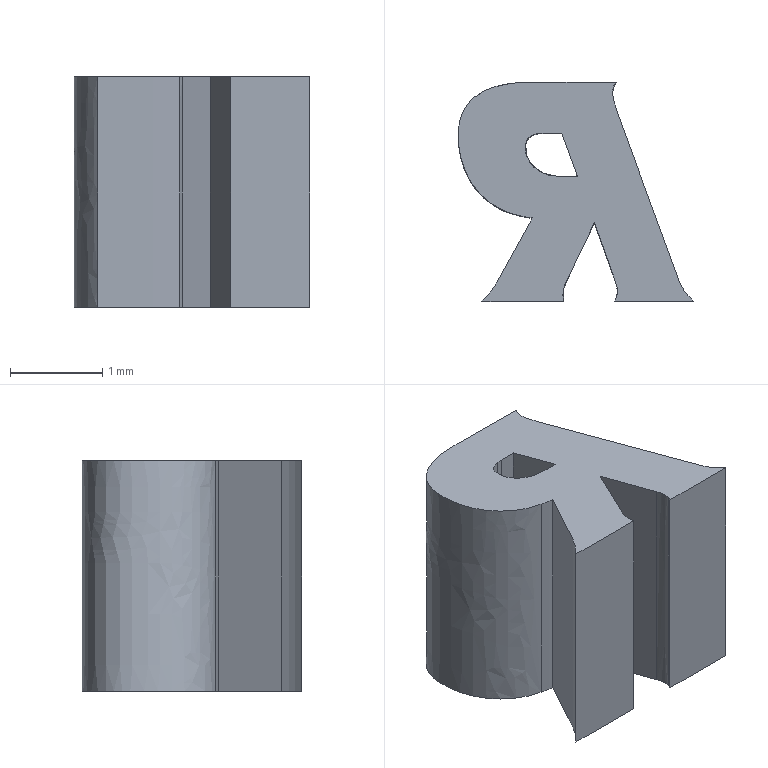Part | STEP file | lll_id1154_x_t | 1 solid | 23 faces | box 2.566 x 2.385 x 2.5 mm | volume 9.126 mm3 | plane 11 | other 7 | cylinder 5 | commonest cylinder face diameters 0.402 x1 1.036 x1 1.606 x1 2.67 x1 71.248 x1
STEP:
#1=CARTESIAN_POINT('',(384.184,124.408,2.35));
#2=VERTEX_POINT('',#1);
#3=CARTESIAN_POINT('',(384.356,123.934,2.35));
#4=VERTEX_POINT('',#3);
#5=CARTESIAN_POINT('',(384.356,123.934,2.35));
#6=DIRECTION('',(0.3416,-0.9399,0.));
#7=VECTOR('',#6,1.);
#8=LINE('',#5,#7);
#9=EDGE_CURVE('',#2,#4,#8,.T.);
#10=ORIENTED_EDGE('',*,*,#9,.F.);
#11=CARTESIAN_POINT('',(384.184,124.408,-0.15));
#12=VERTEX_POINT('',#11);
#13=CARTESIAN_POINT('',(384.184,124.408,-0.15));
#14=DIRECTION('',(0.,0.,-1.));
#15=VECTOR('',#14,1.);
#16=LINE('',#13,#15);
#17=EDGE_CURVE('',#2,#12,#16,.T.);
#18=ORIENTED_EDGE('',*,*,#17,.T.);
#19=CARTESIAN_POINT('',(384.356,123.934,-0.15));
#20=VERTEX_POINT('',#19);
#21=CARTESIAN_POINT('',(384.356,123.934,-0.15));
#22=DIRECTION('',(0.3416,-0.9399,0.));
#23=VECTOR('',#22,1.);
#24=LINE('',#21,#23);
#25=EDGE_CURVE('',#12,#20,#24,.T.);
#26=ORIENTED_EDGE('',*,*,#25,.T.);
#27=CARTESIAN_POINT('',(384.356,123.934,-0.15));
#28=DIRECTION('',(0.,0.,-1.));
#29=VECTOR('',#28,1.);
#30=LINE('',#27,#29);
#31=EDGE_CURVE('',#4,#20,#30,.T.);
#32=ORIENTED_EDGE('',*,*,#31,.F.);
#33=EDGE_LOOP('',(#10,#18,#26,#32));
#34=FACE_OUTER_BOUND('',#33,.T.);
#35=CARTESIAN_POINT('',(384.356,123.934,-0.15));
#36=DIRECTION('',(0.9399,0.3416,0.));
#37=DIRECTION('',(0.3416,-0.9399,0.));
#38=AXIS2_PLACEMENT_3D('',#35,#36,#37);
#39=PLANE('',#38);
#40=ADVANCED_FACE('',(#34),#39,.F.);
#41=CARTESIAN_POINT('',(383.996,124.408,2.35));
#42=VERTEX_POINT('',#41);
#43=CARTESIAN_POINT('',(384.184,124.408,2.35));
#44=DIRECTION('',(1.,0.,0.));
#45=VECTOR('',#44,1.);
#46=LINE('',#43,#45);
#47=EDGE_CURVE('',#42,#2,#46,.T.);
#48=ORIENTED_EDGE('',*,*,#47,.F.);
#49=CARTESIAN_POINT('',(383.996,124.408,-0.15));
#50=VERTEX_POINT('',#49);
#51=CARTESIAN_POINT('',(383.996,124.408,-0.15));
#52=DIRECTION('',(0.,0.,-1.));
#53=VECTOR('',#52,1.);
#54=LINE('',#51,#53);
#55=EDGE_CURVE('',#42,#50,#54,.T.);
#56=ORIENTED_EDGE('',*,*,#55,.T.);
#57=CARTESIAN_POINT('',(384.184,124.408,-0.15));
#58=DIRECTION('',(1.,0.,0.));
#59=VECTOR('',#58,1.);
#60=LINE('',#57,#59);
#61=EDGE_CURVE('',#50,#12,#60,.T.);
#62=ORIENTED_EDGE('',*,*,#61,.T.);
#63=ORIENTED_EDGE('',*,*,#17,.F.);
#64=EDGE_LOOP('',(#48,#56,#62,#63));
#65=FACE_OUTER_BOUND('',#64,.T.);
#66=CARTESIAN_POINT('',(384.184,124.408,-0.15));
#67=DIRECTION('',(0.,1.,0.));
#68=DIRECTION('',(0.,0.,1.));
#69=AXIS2_PLACEMENT_3D('',#66,#67,#68);
#70=PLANE('',#69);
#71=ADVANCED_FACE('',(#65),#70,.F.);
#72=CARTESIAN_POINT('',(383.942,124.405,2.35));
#73=VERTEX_POINT('',#72);
#74=CARTESIAN_POINT('',(383.942,124.405,2.35));
#75=CARTESIAN_POINT('',(383.951,124.406,2.35));
#76=CARTESIAN_POINT('',(383.96,124.407,2.35));
#77=CARTESIAN_POINT('',(383.978,124.408,2.35));
#78=CARTESIAN_POINT('',(383.987,124.408,2.35));
#79=CARTESIAN_POINT('',(383.996,124.408,2.35));
#80=(BOUNDED_CURVE()B_SPLINE_CURVE(3,(#74,#75,#76,#77,#78,#79),.UNSPECIFIED.,.F.,.F.)B_SPLINE_CURVE_WITH_KNOTS((4,2,4),(0.,0.5003,1.),.UNSPECIFIED.)CURVE()GEOMETRIC_REPRESENTATION_ITEM()RATIONAL_B_SPLINE_CURVE((0.5,0.4999,0.4999,0.5,0.5,0.5))REPRESENTATION_ITEM(''));
#81=EDGE_CURVE('',#73,#42,#80,.T.);
#82=ORIENTED_EDGE('',*,*,#81,.F.);
#83=CARTESIAN_POINT('',(383.942,124.405,-0.15));
#84=VERTEX_POINT('',#83);
#85=CARTESIAN_POINT('',(383.942,124.405,-0.15));
#86=DIRECTION('',(0.,0.,-1.));
#87=VECTOR('',#86,1.);
#88=LINE('',#85,#87);
#89=EDGE_CURVE('',#73,#84,#88,.T.);
#90=ORIENTED_EDGE('',*,*,#89,.T.);
#91=CARTESIAN_POINT('',(383.942,124.405,-0.15));
#92=CARTESIAN_POINT('',(383.951,124.406,-0.15));
#93=CARTESIAN_POINT('',(383.96,124.407,-0.15));
#94=CARTESIAN_POINT('',(383.978,124.408,-0.15));
#95=CARTESIAN_POINT('',(383.987,124.408,-0.15));
#96=CARTESIAN_POINT('',(383.996,124.408,-0.15));
#97=(BOUNDED_CURVE()B_SPLINE_CURVE(3,(#91,#92,#93,#94,#95,#96),.UNSPECIFIED.,.F.,.F.)B_SPLINE_CURVE_WITH_KNOTS((4,2,4),(0.,0.5003,1.),.UNSPECIFIED.)CURVE()GEOMETRIC_REPRESENTATION_ITEM()RATIONAL_B_SPLINE_CURVE((0.5,0.4999,0.4999,0.5,0.5,0.5))REPRESENTATION_ITEM(''));
#98=EDGE_CURVE('',#84,#50,#97,.T.);
#99=ORIENTED_EDGE('',*,*,#98,.T.);
#100=ORIENTED_EDGE('',*,*,#55,.F.);
#101=EDGE_LOOP('',(#82,#90,#99,#100));
#102=FACE_OUTER_BOUND('',#101,.T.);
#103=CARTESIAN_POINT('',(383.996,124.408,-0.15));
#104=CARTESIAN_POINT('',(383.987,124.408,-0.15));
#105=CARTESIAN_POINT('',(383.978,124.408,-0.15));
#106=CARTESIAN_POINT('',(383.96,124.407,-0.15));
#107=CARTESIAN_POINT('',(383.951,124.406,-0.15));
#108=CARTESIAN_POINT('',(383.942,124.405,-0.15));
#109=(BOUNDED_CURVE()B_SPLINE_CURVE(3,(#103,#104,#105,#106,#107,#108),.UNSPECIFIED.,.F.,.F.)B_SPLINE_CURVE_WITH_KNOTS((4,2,4),(0.,0.4997,1.),.UNSPECIFIED.)CURVE()GEOMETRIC_REPRESENTATION_ITEM()RATIONAL_B_SPLINE_CURVE((0.5,0.5,0.5,0.4999,0.4999,0.5))REPRESENTATION_ITEM(''));
#110=DIRECTION('',(0.,0.,1.));
#111=VECTOR('',#110,1.);
#112=SURFACE_OF_LINEAR_EXTRUSION('',#109,#111);
#113=ADVANCED_FACE('',(#102),#112,.F.);
#114=CARTESIAN_POINT('',(383.826,124.357,2.35));
#115=VERTEX_POINT('',#114);
#116=CARTESIAN_POINT('',(383.826,124.357,2.35));
#117=CARTESIAN_POINT('',(383.841,124.371,2.35));
#118=CARTESIAN_POINT('',(383.858,124.382,2.35));
#119=CARTESIAN_POINT('',(383.898,124.398,2.35));
#120=CARTESIAN_POINT('',(383.919,124.403,2.35));
#121=CARTESIAN_POINT('',(383.942,124.405,2.35));
#122=(BOUNDED_CURVE()B_SPLINE_CURVE(3,(#116,#117,#118,#119,#120,#121),.UNSPECIFIED.,.F.,.F.)B_SPLINE_CURVE_WITH_KNOTS((4,2,4),(0.,0.4721,1.),.UNSPECIFIED.)CURVE()GEOMETRIC_REPRESENTATION_ITEM()RATIONAL_B_SPLINE_CURVE((0.5,0.4937,0.4937,0.4969,0.4969,0.5))REPRESENTATION_ITEM(''));
#123=EDGE_CURVE('',#115,#73,#122,.T.);
#124=ORIENTED_EDGE('',*,*,#123,.F.);
#125=CARTESIAN_POINT('',(383.826,124.357,-0.15));
#126=VERTEX_POINT('',#125);
#127=CARTESIAN_POINT('',(383.826,124.357,-0.15));
#128=DIRECTION('',(0.,0.,-1.));
#129=VECTOR('',#128,1.);
#130=LINE('',#127,#129);
#131=EDGE_CURVE('',#115,#126,#130,.T.);
#132=ORIENTED_EDGE('',*,*,#131,.T.);
#133=CARTESIAN_POINT('',(383.826,124.357,-0.15));
#134=CARTESIAN_POINT('',(383.841,124.371,-0.15));
#135=CARTESIAN_POINT('',(383.858,124.382,-0.15));
#136=CARTESIAN_POINT('',(383.898,124.398,-0.15));
#137=CARTESIAN_POINT('',(383.919,124.403,-0.15));
#138=CARTESIAN_POINT('',(383.942,124.405,-0.15));
#139=(BOUNDED_CURVE()B_SPLINE_CURVE(3,(#133,#134,#135,#136,#137,#138),.UNSPECIFIED.,.F.,.F.)B_SPLINE_CURVE_WITH_KNOTS((4,2,4),(0.,0.4721,1.),.UNSPECIFIED.)CURVE()GEOMETRIC_REPRESENTATION_ITEM()RATIONAL_B_SPLINE_CURVE((0.5,0.4937,0.4937,0.4969,0.4969,0.5))REPRESENTATION_ITEM(''));
#140=EDGE_CURVE('',#126,#84,#139,.T.);
#141=ORIENTED_EDGE('',*,*,#140,.T.);
#142=ORIENTED_EDGE('',*,*,#89,.F.);
#143=EDGE_LOOP('',(#124,#132,#141,#142));
#144=FACE_OUTER_BOUND('',#143,.T.);
#145=CARTESIAN_POINT('',(383.942,124.405,-0.15));
#146=CARTESIAN_POINT('',(383.919,124.403,-0.15));
#147=CARTESIAN_POINT('',(383.898,124.398,-0.15));
#148=CARTESIAN_POINT('',(383.858,124.382,-0.15));
#149=CARTESIAN_POINT('',(383.841,124.371,-0.15));
#150=CARTESIAN_POINT('',(383.826,124.357,-0.15));
#151=(BOUNDED_CURVE()B_SPLINE_CURVE(3,(#145,#146,#147,#148,#149,#150),.UNSPECIFIED.,.F.,.F.)B_SPLINE_CURVE_WITH_KNOTS((4,2,4),(0.,0.5279,1.),.UNSPECIFIED.)CURVE()GEOMETRIC_REPRESENTATION_ITEM()RATIONAL_B_SPLINE_CURVE((0.5,0.4969,0.4969,0.4937,0.4937,0.5))REPRESENTATION_ITEM(''));
#152=DIRECTION('',(0.,0.,1.));
#153=VECTOR('',#152,1.);
#154=SURFACE_OF_LINEAR_EXTRUSION('',#151,#153);
#155=ADVANCED_FACE('',(#144),#154,.F.);
#156=CARTESIAN_POINT('',(384.178,123.934,2.35));
#157=VERTEX_POINT('',#156);
#158=CARTESIAN_POINT('',(384.178,123.934,2.35));
#159=CARTESIAN_POINT('',(384.16,123.934,2.35));
#160=CARTESIAN_POINT('',(384.142,123.935,2.35));
#161=CARTESIAN_POINT('',(384.102,123.939,2.35));
#162=CARTESIAN_POINT('',(384.08,123.942,2.35));
#163=CARTESIAN_POINT('',(384.032,123.953,2.35));
#164=CARTESIAN_POINT('',(384.007,123.961,2.35));
#165=CARTESIAN_POINT('',(383.945,123.988,2.35));
#166=CARTESIAN_POINT('',(383.912,124.01,2.35));
#167=CARTESIAN_POINT('',(383.842,124.074,2.35));
#168=CARTESIAN_POINT('',(383.814,124.121,2.35));
#169=CARTESIAN_POINT('',(383.791,124.199,2.35));
#170=CARTESIAN_POINT('',(383.787,124.225,2.35));
#171=CARTESIAN_POINT('',(383.787,124.268,2.35));
#172=CARTESIAN_POINT('',(383.789,124.284,2.35));
#173=CARTESIAN_POINT('',(383.799,124.321,2.35));
#174=CARTESIAN_POINT('',(383.81,124.341,2.35));
#175=CARTESIAN_POINT('',(383.826,124.357,2.35));
#176=(BOUNDED_CURVE()B_SPLINE_CURVE(3,(#158,#159,#160,#161,#162,#163,#164,#165,#166,#167,#168,#169,#170,#171,#172,#173,#174,#175),.UNSPECIFIED.,.F.,.F.)B_SPLINE_CURVE_WITH_KNOTS((4,2,2,2,2,2,2,2,4),(0.,0.07697,0.1735,0.2892,0.4651,0.7036,0.825,0.8964,1.),.UNSPECIFIED.)CURVE()GEOMETRIC_REPRESENTATION_ITEM()RATIONAL_B_SPLINE_CURVE((0.5,0.4998,0.4998,0.4994,0.4994,0.4983,0.4983,0.4952,0.4952,0.4878,0.4878,0.4966,0.4966,0.4974,0.4974,0.4878,0.4878,0.5))REPRESENTATION_ITEM(''));
#177=EDGE_CURVE('',#157,#115,#176,.T.);
#178=ORIENTED_EDGE('',*,*,#177,.F.);
#179=CARTESIAN_POINT('',(384.178,123.934,-0.15));
#180=VERTEX_POINT('',#179);
#181=CARTESIAN_POINT('',(384.178,123.934,-0.15));
#182=DIRECTION('',(0.,0.,-1.));
#183=VECTOR('',#182,1.);
#184=LINE('',#181,#183);
#185=EDGE_CURVE('',#157,#180,#184,.T.);
#186=ORIENTED_EDGE('',*,*,#185,.T.);
#187=CARTESIAN_POINT('',(384.178,123.934,-0.15));
#188=CARTESIAN_POINT('',(384.16,123.934,-0.15));
#189=CARTESIAN_POINT('',(384.142,123.935,-0.15));
#190=CARTESIAN_POINT('',(384.102,123.939,-0.15));
#191=CARTESIAN_POINT('',(384.08,123.942,-0.15));
#192=CARTESIAN_POINT('',(384.032,123.953,-0.15));
#193=CARTESIAN_POINT('',(384.007,123.961,-0.15));
#194=CARTESIAN_POINT('',(383.945,123.988,-0.15));
#195=CARTESIAN_POINT('',(383.912,124.01,-0.15));
#196=CARTESIAN_POINT('',(383.842,124.074,-0.15));
#197=CARTESIAN_POINT('',(383.814,124.121,-0.15));
#198=CARTESIAN_POINT('',(383.791,124.199,-0.15));
#199=CARTESIAN_POINT('',(383.787,124.225,-0.15));
#200=CARTESIAN_POINT('',(383.787,124.268,-0.15));
#201=CARTESIAN_POINT('',(383.789,124.284,-0.15));
#202=CARTESIAN_POINT('',(383.799,124.321,-0.15));
#203=CARTESIAN_POINT('',(383.81,124.341,-0.15));
#204=CARTESIAN_POINT('',(383.826,124.357,-0.15));
#205=(BOUNDED_CURVE()B_SPLINE_CURVE(3,(#187,#188,#189,#190,#191,#192,#193,#194,#195,#196,#197,#198,#199,#200,#201,#202,#203,#204),.UNSPECIFIED.,.F.,.F.)B_SPLINE_CURVE_WITH_KNOTS((4,2,2,2,2,2,2,2,4),(0.,0.07697,0.1735,0.2892,0.4651,0.7036,0.825,0.8964,1.),.UNSPECIFIED.)CURVE()GEOMETRIC_REPRESENTATION_ITEM()RATIONAL_B_SPLINE_CURVE((0.5,0.4998,0.4998,0.4994,0.4994,0.4983,0.4983,0.4952,0.4952,0.4878,0.4878,0.4966,0.4966,0.4974,0.4974,0.4878,0.4878,0.5))REPRESENTATION_ITEM(''));
#206=EDGE_CURVE('',#180,#126,#205,.T.);
#207=ORIENTED_EDGE('',*,*,#206,.T.);
#208=ORIENTED_EDGE('',*,*,#131,.F.);
#209=EDGE_LOOP('',(#178,#186,#207,#208));
#210=FACE_OUTER_BOUND('',#209,.T.);
#211=CARTESIAN_POINT('',(383.826,124.357,-0.15));
#212=CARTESIAN_POINT('',(383.81,124.341,-0.15));
#213=CARTESIAN_POINT('',(383.799,124.321,-0.15));
#214=CARTESIAN_POINT('',(383.789,124.284,-0.15));
#215=CARTESIAN_POINT('',(383.787,124.268,-0.15));
#216=CARTESIAN_POINT('',(383.787,124.225,-0.15));
#217=CARTESIAN_POINT('',(383.791,124.199,-0.15));
#218=CARTESIAN_POINT('',(383.814,124.121,-0.15));
#219=CARTESIAN_POINT('',(383.842,124.074,-0.15));
#220=CARTESIAN_POINT('',(383.912,124.01,-0.15));
#221=CARTESIAN_POINT('',(383.945,123.988,-0.15));
#222=CARTESIAN_POINT('',(384.007,123.961,-0.15));
#223=CARTESIAN_POINT('',(384.032,123.953,-0.15));
#224=CARTESIAN_POINT('',(384.08,123.942,-0.15));
#225=CARTESIAN_POINT('',(384.102,123.939,-0.15));
#226=CARTESIAN_POINT('',(384.142,123.935,-0.15));
#227=CARTESIAN_POINT('',(384.16,123.934,-0.15));
#228=CARTESIAN_POINT('',(384.178,123.934,-0.15));
#229=(BOUNDED_CURVE()B_SPLINE_CURVE(3,(#211,#212,#213,#214,#215,#216,#217,#218,#219,#220,#221,#222,#223,#224,#225,#226,#227,#228),.UNSPECIFIED.,.F.,.F.)B_SPLINE_CURVE_WITH_KNOTS((4,2,2,2,2,2,2,2,4),(0.,0.1036,0.175,0.2964,0.5349,0.7108,0.8265,0.923,1.),.UNSPECIFIED.)CURVE()GEOMETRIC_REPRESENTATION_ITEM()RATIONAL_B_SPLINE_CURVE((0.5,0.4878,0.4878,0.4974,0.4974,0.4966,0.4966,0.4878,0.4878,0.4952,0.4952,0.4983,0.4983,0.4994,0.4994,0.4998,0.4998,0.5))REPRESENTATION_ITEM(''));
#230=DIRECTION('',(0.,0.,1.));
#231=VECTOR('',#230,1.);
#232=SURFACE_OF_LINEAR_EXTRUSION('',#229,#231);
#233=ADVANCED_FACE('',(#210),#232,.F.);
#234=CARTESIAN_POINT('',(385.618,122.58,2.35));
#235=VERTEX_POINT('',#234);
#236=CARTESIAN_POINT('',(385.461,122.794,2.35));
#237=VERTEX_POINT('',#236);
#238=CARTESIAN_POINT('',(385.942,122.987,2.35));
#239=DIRECTION('',(0.,0.,-1.));
#240=DIRECTION('',(-1.,0.,0.));
#241=AXIS2_PLACEMENT_3D('',#238,#239,#240);
#242=CIRCLE('',#241,0.5179);
#243=EDGE_CURVE('',#235,#237,#242,.T.);
#244=ORIENTED_EDGE('',*,*,#243,.F.);
#245=CARTESIAN_POINT('',(385.618,122.58,-0.15));
#246=VERTEX_POINT('',#245);
#247=CARTESIAN_POINT('',(385.624,122.578,2.35));
#248=DIRECTION('',(0.,0.,-1.));
#249=VECTOR('',#248,1.);
#250=LINE('',#247,#249);
#251=EDGE_CURVE('',#235,#246,#250,.T.);
#252=ORIENTED_EDGE('',*,*,#251,.T.);
#253=CARTESIAN_POINT('',(385.461,122.794,-0.15));
#254=VERTEX_POINT('',#253);
#255=CARTESIAN_POINT('',(385.942,122.987,-0.15));
#256=DIRECTION('',(0.,0.,-1.));
#257=DIRECTION('',(-1.,0.,0.));
#258=AXIS2_PLACEMENT_3D('',#255,#256,#257);
#259=CIRCLE('',#258,0.5179);
#260=EDGE_CURVE('',#246,#254,#259,.T.);
#261=ORIENTED_EDGE('',*,*,#260,.T.);
#262=CARTESIAN_POINT('',(385.461,122.794,-0.15));
#263=DIRECTION('',(0.,0.,-1.));
#264=VECTOR('',#263,1.);
#265=LINE('',#262,#264);
#266=EDGE_CURVE('',#237,#254,#265,.T.);
#267=ORIENTED_EDGE('',*,*,#266,.F.);
#268=EDGE_LOOP('',(#244,#252,#261,#267));
#269=FACE_OUTER_BOUND('',#268,.T.);
#270=CARTESIAN_POINT('',(385.942,122.987,-0.15));
#271=DIRECTION('',(0.,0.,1.));
#272=DIRECTION('',(1.,0.,0.));
#273=AXIS2_PLACEMENT_3D('',#270,#271,#272);
#274=CYLINDRICAL_SURFACE('',#273,0.5179);
#275=ADVANCED_FACE('',(#269),#274,.F.);
#276=CARTESIAN_POINT('',(384.758,122.58,2.35));
#277=VERTEX_POINT('',#276);
#278=CARTESIAN_POINT('',(385.618,122.578,2.35));
#279=DIRECTION('',(1.,0.,0.));
#280=VECTOR('',#279,1.);
#281=LINE('',#278,#280);
#282=EDGE_CURVE('',#277,#235,#281,.T.);
#283=ORIENTED_EDGE('',*,*,#282,.F.);
#284=CARTESIAN_POINT('',(384.758,122.58,-0.15));
#285=VERTEX_POINT('',#284);
#286=CARTESIAN_POINT('',(384.754,122.578,2.35));
#287=DIRECTION('',(0.,0.,-1.));
#288=VECTOR('',#287,1.);
#289=LINE('',#286,#288);
#290=EDGE_CURVE('',#277,#285,#289,.T.);
#291=ORIENTED_EDGE('',*,*,#290,.T.);
#292=CARTESIAN_POINT('',(385.618,122.578,-0.15));
#293=DIRECTION('',(1.,0.,0.));
#294=VECTOR('',#293,1.);
#295=LINE('',#292,#294);
#296=EDGE_CURVE('',#285,#246,#295,.T.);
#297=ORIENTED_EDGE('',*,*,#296,.T.);
#298=ORIENTED_EDGE('',*,*,#251,.F.);
#299=EDGE_LOOP('',(#283,#291,#297,#298));
#300=FACE_OUTER_BOUND('',#299,.T.);
#301=CARTESIAN_POINT('',(385.618,122.578,-0.15));
#302=DIRECTION('',(0.,1.,0.));
#303=DIRECTION('',(0.,0.,1.));
#304=AXIS2_PLACEMENT_3D('',#301,#302,#303);
#305=PLANE('',#304);
#306=ADVANCED_FACE('',(#300),#305,.F.);
#307=CARTESIAN_POINT('',(384.778,122.622,2.35));
#308=VERTEX_POINT('',#307);
#309=CARTESIAN_POINT('',(384.778,122.622,2.35));
#310=CARTESIAN_POINT('',(384.773,122.608,2.35));
#311=CARTESIAN_POINT('',(384.766,122.595,2.35));
#312=CARTESIAN_POINT('',(384.758,122.583,2.35));
#313=(BOUNDED_CURVE()B_SPLINE_CURVE(3,(#309,#310,#311,#312),.UNSPECIFIED.,.F.,.F.)B_SPLINE_CURVE_WITH_KNOTS((4,4),(0.,1.),.UNSPECIFIED.)CURVE()GEOMETRIC_REPRESENTATION_ITEM()RATIONAL_B_SPLINE_CURVE((0.5015,0.4995,0.4995,0.5015))REPRESENTATION_ITEM(''));
#314=EDGE_CURVE('',#308,#277,#313,.T.);
#315=ORIENTED_EDGE('',*,*,#314,.F.);
#316=CARTESIAN_POINT('',(384.778,122.622,-0.15));
#317=VERTEX_POINT('',#316);
#318=CARTESIAN_POINT('',(384.778,122.622,-0.15));
#319=DIRECTION('',(0.,0.,-1.));
#320=VECTOR('',#319,1.);
#321=LINE('',#318,#320);
#322=EDGE_CURVE('',#308,#317,#321,.T.);
#323=ORIENTED_EDGE('',*,*,#322,.T.);
#324=CARTESIAN_POINT('',(384.778,122.622,-0.15));
#325=CARTESIAN_POINT('',(384.773,122.608,-0.15));
#326=CARTESIAN_POINT('',(384.766,122.595,-0.15));
#327=CARTESIAN_POINT('',(384.758,122.583,-0.15));
#328=(BOUNDED_CURVE()B_SPLINE_CURVE(3,(#324,#325,#326,#327),.UNSPECIFIED.,.F.,.F.)B_SPLINE_CURVE_WITH_KNOTS((4,4),(0.,1.),.UNSPECIFIED.)CURVE()GEOMETRIC_REPRESENTATION_ITEM()RATIONAL_B_SPLINE_CURVE((0.5015,0.4995,0.4995,0.5015))REPRESENTATION_ITEM(''));
#329=EDGE_CURVE('',#317,#285,#328,.T.);
#330=ORIENTED_EDGE('',*,*,#329,.T.);
#331=ORIENTED_EDGE('',*,*,#290,.F.);
#332=EDGE_LOOP('',(#315,#323,#330,#331));
#333=FACE_OUTER_BOUND('',#332,.T.);
#334=CARTESIAN_POINT('',(384.592,122.696,-0.15));
#335=DIRECTION('',(0.,0.,1.));
#336=DIRECTION('',(1.,0.,0.));
#337=AXIS2_PLACEMENT_3D('',#334,#335,#336);
#338=CYLINDRICAL_SURFACE('',#337,0.2008);
#339=ADVANCED_FACE('',(#333),#338,.F.);
#340=CARTESIAN_POINT('',(384.769,122.789,2.35));
#341=VERTEX_POINT('',#340);
#342=CARTESIAN_POINT('',(384.769,122.789,2.35));
#343=CARTESIAN_POINT('',(384.772,122.779,2.35));
#344=CARTESIAN_POINT('',(384.776,122.768,2.35));
#345=CARTESIAN_POINT('',(384.782,122.747,2.35));
#346=CARTESIAN_POINT('',(384.784,122.736,2.35));
#347=CARTESIAN_POINT('',(384.788,122.713,2.35));
#348=CARTESIAN_POINT('',(384.789,122.702,2.35));
#349=CARTESIAN_POINT('',(384.79,122.684,2.35));
#350=CARTESIAN_POINT('',(384.79,122.678,2.35));
#351=CARTESIAN_POINT('',(384.788,122.654,2.35));
#352=CARTESIAN_POINT('',(384.784,122.637,2.35));
#353=CARTESIAN_POINT('',(384.778,122.622,2.35));
#354=(BOUNDED_CURVE()B_SPLINE_CURVE(3,(#342,#343,#344,#345,#346,#347,#348,#349,#350,#351,#352,#353),.UNSPECIFIED.,.F.,.F.)B_SPLINE_CURVE_WITH_KNOTS((4,2,2,2,2,4),(0.,0.1952,0.3909,0.5862,0.7038,1.),.UNSPECIFIED.)CURVE()GEOMETRIC_REPRESENTATION_ITEM()RATIONAL_B_SPLINE_CURVE((0.5015,0.5013,0.5013,0.5011,0.5011,0.5007,0.5007,0.5011,0.5011,0.4976,0.4976,0.5015))REPRESENTATION_ITEM(''));
#355=EDGE_CURVE('',#341,#308,#354,.T.);
#356=ORIENTED_EDGE('',*,*,#355,.F.);
#357=CARTESIAN_POINT('',(384.769,122.789,-0.15));
#358=VERTEX_POINT('',#357);
#359=CARTESIAN_POINT('',(384.769,122.789,-0.15));
#360=DIRECTION('',(0.,0.,-1.));
#361=VECTOR('',#360,1.);
#362=LINE('',#359,#361);
#363=EDGE_CURVE('',#341,#358,#362,.T.);
#364=ORIENTED_EDGE('',*,*,#363,.T.);
#365=CARTESIAN_POINT('',(384.769,122.789,-0.15));
#366=CARTESIAN_POINT('',(384.772,122.779,-0.15));
#367=CARTESIAN_POINT('',(384.776,122.768,-0.15));
#368=CARTESIAN_POINT('',(384.782,122.747,-0.15));
#369=CARTESIAN_POINT('',(384.784,122.736,-0.15));
#370=CARTESIAN_POINT('',(384.788,122.713,-0.15));
#371=CARTESIAN_POINT('',(384.789,122.702,-0.15));
#372=CARTESIAN_POINT('',(384.79,122.684,-0.15));
#373=CARTESIAN_POINT('',(384.79,122.678,-0.15));
#374=CARTESIAN_POINT('',(384.788,122.654,-0.15));
#375=CARTESIAN_POINT('',(384.784,122.637,-0.15));
#376=CARTESIAN_POINT('',(384.778,122.622,-0.15));
#377=(BOUNDED_CURVE()B_SPLINE_CURVE(3,(#365,#366,#367,#368,#369,#370,#371,#372,#373,#374,#375,#376),.UNSPECIFIED.,.F.,.F.)B_SPLINE_CURVE_WITH_KNOTS((4,2,2,2,2,4),(0.,0.1952,0.3909,0.5862,0.7038,1.),.UNSPECIFIED.)CURVE()GEOMETRIC_REPRESENTATION_ITEM()RATIONAL_B_SPLINE_CURVE((0.5015,0.5013,0.5013,0.5011,0.5011,0.5007,0.5007,0.5011,0.5011,0.4976,0.4976,0.5015))REPRESENTATION_ITEM(''));
#378=EDGE_CURVE('',#358,#317,#377,.T.);
#379=ORIENTED_EDGE('',*,*,#378,.T.);
#380=ORIENTED_EDGE('',*,*,#322,.F.);
#381=EDGE_LOOP('',(#356,#364,#379,#380));
#382=FACE_OUTER_BOUND('',#381,.T.);
#383=CARTESIAN_POINT('',(384.778,122.622,-0.15));
#384=CARTESIAN_POINT('',(384.784,122.637,-0.15));
#385=CARTESIAN_POINT('',(384.788,122.654,-0.15));
#386=CARTESIAN_POINT('',(384.79,122.678,-0.15));
#387=CARTESIAN_POINT('',(384.79,122.684,-0.15));
#388=CARTESIAN_POINT('',(384.789,122.702,-0.15));
#389=CARTESIAN_POINT('',(384.788,122.713,-0.15));
#390=CARTESIAN_POINT('',(384.784,122.736,-0.15));
#391=CARTESIAN_POINT('',(384.782,122.747,-0.15));
#392=CARTESIAN_POINT('',(384.776,122.768,-0.15));
#393=CARTESIAN_POINT('',(384.772,122.779,-0.15));
#394=CARTESIAN_POINT('',(384.769,122.789,-0.15));
#395=(BOUNDED_CURVE()B_SPLINE_CURVE(3,(#383,#384,#385,#386,#387,#388,#389,#390,#391,#392,#393,#394),.UNSPECIFIED.,.F.,.F.)B_SPLINE_CURVE_WITH_KNOTS((4,2,2,2,2,4),(0.,0.2962,0.4138,0.6091,0.8048,1.),.UNSPECIFIED.)CURVE()GEOMETRIC_REPRESENTATION_ITEM()RATIONAL_B_SPLINE_CURVE((0.5015,0.4976,0.4976,0.5011,0.5011,0.5007,0.5007,0.5011,0.5011,0.5013,0.5013,0.5015))REPRESENTATION_ITEM(''));
#396=DIRECTION('',(0.,0.,1.));
#397=VECTOR('',#396,1.);
#398=SURFACE_OF_LINEAR_EXTRUSION('',#395,#397);
#399=ADVANCED_FACE('',(#382),#398,.F.);
#400=CARTESIAN_POINT('',(384.539,123.432,2.35));
#401=VERTEX_POINT('',#400);
#402=CARTESIAN_POINT('',(384.769,122.789,2.35));
#403=DIRECTION('',(0.337,-0.9415,0.));
#404=VECTOR('',#403,1.);
#405=LINE('',#402,#404);
#406=EDGE_CURVE('',#401,#341,#405,.T.);
#407=ORIENTED_EDGE('',*,*,#406,.F.);
#408=CARTESIAN_POINT('',(384.539,123.432,-0.15));
#409=VERTEX_POINT('',#408);
#410=CARTESIAN_POINT('',(384.539,123.432,-0.15));
#411=DIRECTION('',(0.,0.,-1.));
#412=VECTOR('',#411,1.);
#413=LINE('',#410,#412);
#414=EDGE_CURVE('',#401,#409,#413,.T.);
#415=ORIENTED_EDGE('',*,*,#414,.T.);
#416=CARTESIAN_POINT('',(384.769,122.789,-0.15));
#417=DIRECTION('',(0.337,-0.9415,0.));
#418=VECTOR('',#417,1.);
#419=LINE('',#416,#418);
#420=EDGE_CURVE('',#409,#358,#419,.T.);
#421=ORIENTED_EDGE('',*,*,#420,.T.);
#422=ORIENTED_EDGE('',*,*,#363,.F.);
#423=EDGE_LOOP('',(#407,#415,#421,#422));
#424=FACE_OUTER_BOUND('',#423,.T.);
#425=CARTESIAN_POINT('',(384.769,122.789,-0.15));
#426=DIRECTION('',(0.9415,0.337,0.));
#427=DIRECTION('',(0.337,-0.9415,0.));
#428=AXIS2_PLACEMENT_3D('',#425,#426,#427);
#429=PLANE('',#428);
#430=ADVANCED_FACE('',(#424),#429,.F.);
#431=CARTESIAN_POINT('',(384.233,122.793,2.35));
#432=VERTEX_POINT('',#431);
#433=CARTESIAN_POINT('',(384.539,123.432,2.35));
#434=DIRECTION('',(0.4316,0.902,0.));
#435=VECTOR('',#434,1.);
#436=LINE('',#433,#435);
#437=EDGE_CURVE('',#432,#401,#436,.T.);
#438=ORIENTED_EDGE('',*,*,#437,.F.);
#439=CARTESIAN_POINT('',(384.233,122.793,-0.15));
#440=VERTEX_POINT('',#439);
#441=CARTESIAN_POINT('',(384.233,122.793,-0.15));
#442=DIRECTION('',(0.,0.,-1.));
#443=VECTOR('',#442,1.);
#444=LINE('',#441,#443);
#445=EDGE_CURVE('',#432,#440,#444,.T.);
#446=ORIENTED_EDGE('',*,*,#445,.T.);
#447=CARTESIAN_POINT('',(384.539,123.432,-0.15));
#448=DIRECTION('',(0.4316,0.902,0.));
#449=VECTOR('',#448,1.);
#450=LINE('',#447,#449);
#451=EDGE_CURVE('',#440,#409,#450,.T.);
#452=ORIENTED_EDGE('',*,*,#451,.T.);
#453=ORIENTED_EDGE('',*,*,#414,.F.);
#454=EDGE_LOOP('',(#438,#446,#452,#453));
#455=FACE_OUTER_BOUND('',#454,.T.);
#456=CARTESIAN_POINT('',(384.539,123.432,-0.15));
#457=DIRECTION('',(-0.902,0.4316,0.));
#458=DIRECTION('',(0.4316,0.902,0.));
#459=AXIS2_PLACEMENT_3D('',#456,#457,#458);
#460=PLANE('',#459);
#461=ADVANCED_FACE('',(#455),#460,.F.);
#462=CARTESIAN_POINT('',(384.206,122.58,2.35));
#463=VERTEX_POINT('',#462);
#464=CARTESIAN_POINT('',(384.205,122.581,2.35));
#465=CARTESIAN_POINT('',(384.202,122.592,2.35));
#466=CARTESIAN_POINT('',(384.2,122.603,2.35));
#467=CARTESIAN_POINT('',(384.197,122.626,2.35));
#468=CARTESIAN_POINT('',(384.196,122.637,2.35));
#469=CARTESIAN_POINT('',(384.196,122.665,2.35));
#470=CARTESIAN_POINT('',(384.197,122.68,2.35));
#471=CARTESIAN_POINT('',(384.203,122.712,2.35));
#472=CARTESIAN_POINT('',(384.207,122.727,2.35));
#473=CARTESIAN_POINT('',(384.218,122.76,2.35));
#474=CARTESIAN_POINT('',(384.225,122.777,2.35));
#475=CARTESIAN_POINT('',(384.233,122.793,2.35));
#476=(BOUNDED_CURVE()B_SPLINE_CURVE(3,(#464,#465,#466,#467,#468,#469,#470,#471,#472,#473,#474,#475),.UNSPECIFIED.,.F.,.F.)B_SPLINE_CURVE_WITH_KNOTS((4,2,2,2,2,4),(0.,0.156,0.3115,0.5302,0.749,1.),.UNSPECIFIED.)CURVE()GEOMETRIC_REPRESENTATION_ITEM()RATIONAL_B_SPLINE_CURVE((0.5005,0.4999,0.4999,0.4995,0.4995,0.4991,0.4991,0.4996,0.4996,0.4998,0.4998,0.5005))REPRESENTATION_ITEM(''));
#477=EDGE_CURVE('',#463,#432,#476,.T.);
#478=ORIENTED_EDGE('',*,*,#477,.F.);
#479=CARTESIAN_POINT('',(384.206,122.58,-0.15));
#480=VERTEX_POINT('',#479);
#481=CARTESIAN_POINT('',(384.206,122.578,2.35));
#482=DIRECTION('',(0.,0.,-1.));
#483=VECTOR('',#482,1.);
#484=LINE('',#481,#483);
#485=EDGE_CURVE('',#463,#480,#484,.T.);
#486=ORIENTED_EDGE('',*,*,#485,.T.);
#487=CARTESIAN_POINT('',(384.206,122.579,-0.15));
#488=CARTESIAN_POINT('',(384.206,122.58,-0.15));
#489=CARTESIAN_POINT('',(384.206,122.581,-0.15));
#490=CARTESIAN_POINT('',(384.202,122.592,-0.15));
#491=CARTESIAN_POINT('',(384.2,122.603,-0.15));
#492=CARTESIAN_POINT('',(384.197,122.626,-0.15));
#493=CARTESIAN_POINT('',(384.196,122.637,-0.15));
#494=CARTESIAN_POINT('',(384.196,122.665,-0.15));
#495=CARTESIAN_POINT('',(384.197,122.68,-0.15));
#496=CARTESIAN_POINT('',(384.203,122.712,-0.15));
#497=CARTESIAN_POINT('',(384.207,122.727,-0.15));
#498=CARTESIAN_POINT('',(384.218,122.76,-0.15));
#499=CARTESIAN_POINT('',(384.225,122.777,-0.15));
#500=CARTESIAN_POINT('',(384.233,122.793,-0.15));
#501=(BOUNDED_CURVE()B_SPLINE_CURVE(3,(#487,#488,#489,#490,#491,#492,#493,#494,#495,#496,#497,#498,#499,#500),.UNSPECIFIED.,.F.,.F.)B_SPLINE_CURVE_WITH_KNOTS((4,2,2,2,2,2,4),(0.,0.009901,0.1643,0.3183,0.5348,0.7515,1.),.UNSPECIFIED.)CURVE()GEOMETRIC_REPRESENTATION_ITEM()RATIONAL_B_SPLINE_CURVE((0.5005,0.5005,0.5005,0.4999,0.4999,0.4995,0.4995,0.4991,0.4991,0.4996,0.4996,0.4998,0.4998,0.5005))REPRESENTATION_ITEM(''));
#502=EDGE_CURVE('',#480,#440,#501,.T.);
#503=ORIENTED_EDGE('',*,*,#502,.T.);
#504=ORIENTED_EDGE('',*,*,#445,.F.);
#505=EDGE_LOOP('',(#478,#486,#503,#504));
#506=FACE_OUTER_BOUND('',#505,.T.);
#507=CARTESIAN_POINT('',(384.233,122.793,-0.15));
#508=CARTESIAN_POINT('',(384.225,122.777,-0.15));
#509=CARTESIAN_POINT('',(384.218,122.76,-0.15));
#510=CARTESIAN_POINT('',(384.207,122.727,-0.15));
#511=CARTESIAN_POINT('',(384.203,122.712,-0.15));
#512=CARTESIAN_POINT('',(384.197,122.68,-0.15));
#513=CARTESIAN_POINT('',(384.196,122.665,-0.15));
#514=CARTESIAN_POINT('',(384.196,122.637,-0.15));
#515=CARTESIAN_POINT('',(384.197,122.626,-0.15));
#516=CARTESIAN_POINT('',(384.2,122.603,-0.15));
#517=CARTESIAN_POINT('',(384.202,122.592,-0.15));
#518=CARTESIAN_POINT('',(384.206,122.581,-0.15));
#519=CARTESIAN_POINT('',(384.206,122.58,-0.15));
#520=CARTESIAN_POINT('',(384.206,122.578,-0.15));
#521=CARTESIAN_POINT('',(384.206,122.578,-0.15));
#522=CARTESIAN_POINT('',(384.207,122.577,-0.15));
#523=(BOUNDED_CURVE()B_SPLINE_CURVE(3,(#507,#508,#509,#510,#511,#512,#513,#514,#515,#516,#517,#518,#519,#520,#521,#522),.UNSPECIFIED.,.F.,.F.)B_SPLINE_CURVE_WITH_KNOTS((4,2,2,2,2,2,2,4),(0.,0.246,0.4605,0.6749,0.8274,0.9803,0.9901,1.),.UNSPECIFIED.)CURVE()GEOMETRIC_REPRESENTATION_ITEM()RATIONAL_B_SPLINE_CURVE((0.5005,0.4998,0.4998,0.4996,0.4996,0.4991,0.4991,0.4995,0.4995,0.4999,0.4999,0.5005,0.5005,0.5005,0.5005,0.5005))REPRESENTATION_ITEM(''));
#524=DIRECTION('',(0.,0.,1.));
#525=VECTOR('',#524,1.);
#526=SURFACE_OF_LINEAR_EXTRUSION('',#523,#525);
#527=ADVANCED_FACE('',(#506),#526,.F.);
#528=CARTESIAN_POINT('',(383.316,122.583,2.35));
#529=VERTEX_POINT('',#528);
#530=CARTESIAN_POINT('',(383.973,158.201,2.35));
#531=DIRECTION('',(0.,0.,1.));
#532=DIRECTION('',(-1.,0.,0.));
#533=AXIS2_PLACEMENT_3D('',#530,#531,#532);
#534=CIRCLE('',#533,35.624);
#535=EDGE_CURVE('',#529,#463,#534,.T.);
#536=ORIENTED_EDGE('',*,*,#535,.F.);
#537=CARTESIAN_POINT('',(383.316,122.583,-0.15));
#538=VERTEX_POINT('',#537);
#539=CARTESIAN_POINT('',(383.316,122.583,-0.15));
#540=DIRECTION('',(0.,0.,-1.));
#541=VECTOR('',#540,1.);
#542=LINE('',#539,#541);
#543=EDGE_CURVE('',#529,#538,#542,.T.);
#544=ORIENTED_EDGE('',*,*,#543,.T.);
#545=CARTESIAN_POINT('',(383.973,158.201,-0.15));
#546=DIRECTION('',(0.,0.,1.));
#547=DIRECTION('',(-1.,0.,0.));
#548=AXIS2_PLACEMENT_3D('',#545,#546,#547);
#549=CIRCLE('',#548,35.624);
#550=EDGE_CURVE('',#538,#480,#549,.T.);
#551=ORIENTED_EDGE('',*,*,#550,.T.);
#552=ORIENTED_EDGE('',*,*,#485,.F.);
#553=EDGE_LOOP('',(#536,#544,#551,#552));
#554=FACE_OUTER_BOUND('',#553,.T.);
#555=CARTESIAN_POINT('',(383.973,158.201,-0.15));
#556=DIRECTION('',(0.,0.,1.));
#557=DIRECTION('',(1.,0.,0.));
#558=AXIS2_PLACEMENT_3D('',#555,#556,#557);
#559=CYLINDRICAL_SURFACE('',#558,35.624);
#560=ADVANCED_FACE('',(#554),#559,.T.);
#561=CARTESIAN_POINT('',(383.484,122.793,2.35));
#562=VERTEX_POINT('',#561);
#563=CARTESIAN_POINT('',(382.782,123.182,2.35));
#564=DIRECTION('',(0.,0.,-1.));
#565=DIRECTION('',(-1.,0.,0.));
#566=AXIS2_PLACEMENT_3D('',#563,#564,#565);
#567=CIRCLE('',#566,0.8029);
#568=EDGE_CURVE('',#562,#529,#567,.T.);
#569=ORIENTED_EDGE('',*,*,#568,.F.);
#570=CARTESIAN_POINT('',(383.484,122.793,-0.15));
#571=VERTEX_POINT('',#570);
#572=CARTESIAN_POINT('',(383.484,122.793,-0.15));
#573=DIRECTION('',(0.,0.,-1.));
#574=VECTOR('',#573,1.);
#575=LINE('',#572,#574);
#576=EDGE_CURVE('',#562,#571,#575,.T.);
#577=ORIENTED_EDGE('',*,*,#576,.T.);
#578=CARTESIAN_POINT('',(382.782,123.182,-0.15));
#579=DIRECTION('',(0.,0.,-1.));
#580=DIRECTION('',(-1.,0.,0.));
#581=AXIS2_PLACEMENT_3D('',#578,#579,#580);
#582=CIRCLE('',#581,0.8029);
#583=EDGE_CURVE('',#571,#538,#582,.T.);
#584=ORIENTED_EDGE('',*,*,#583,.T.);
#585=ORIENTED_EDGE('',*,*,#543,.F.);
#586=EDGE_LOOP('',(#569,#577,#584,#585));
#587=FACE_OUTER_BOUND('',#586,.T.);
#588=CARTESIAN_POINT('',(382.782,123.182,-0.15));
#589=DIRECTION('',(0.,0.,1.));
#590=DIRECTION('',(1.,0.,0.));
#591=AXIS2_PLACEMENT_3D('',#588,#589,#590);
#592=CYLINDRICAL_SURFACE('',#591,0.8029);
#593=ADVANCED_FACE('',(#587),#592,.F.);
#594=CARTESIAN_POINT('',(383.864,123.485,2.35));
#595=VERTEX_POINT('',#594);
#596=CARTESIAN_POINT('',(383.484,122.793,2.35));
#597=DIRECTION('',(-0.4811,-0.8767,0.));
#598=VECTOR('',#597,1.);
#599=LINE('',#596,#598);
#600=EDGE_CURVE('',#595,#562,#599,.T.);
#601=ORIENTED_EDGE('',*,*,#600,.F.);
#602=CARTESIAN_POINT('',(383.864,123.485,-0.15));
#603=VERTEX_POINT('',#602);
#604=CARTESIAN_POINT('',(383.864,123.485,-0.15));
#605=DIRECTION('',(0.,0.,-1.));
#606=VECTOR('',#605,1.);
#607=LINE('',#604,#606);
#608=EDGE_CURVE('',#595,#603,#607,.T.);
#609=ORIENTED_EDGE('',*,*,#608,.T.);
#610=CARTESIAN_POINT('',(383.484,122.793,-0.15));
#611=DIRECTION('',(-0.4811,-0.8767,0.));
#612=VECTOR('',#611,1.);
#613=LINE('',#610,#612);
#614=EDGE_CURVE('',#603,#571,#613,.T.);
#615=ORIENTED_EDGE('',*,*,#614,.T.);
#616=ORIENTED_EDGE('',*,*,#576,.F.);
#617=EDGE_LOOP('',(#601,#609,#615,#616));
#618=FACE_OUTER_BOUND('',#617,.T.);
#619=CARTESIAN_POINT('',(383.484,122.793,-0.15));
#620=DIRECTION('',(0.8767,-0.4811,0.));
#621=DIRECTION('',(-0.4811,-0.8767,0.));
#622=AXIS2_PLACEMENT_3D('',#619,#620,#621);
#623=PLANE('',#622);
#624=ADVANCED_FACE('',(#618),#623,.F.);
#625=CARTESIAN_POINT('',(383.712,123.512,2.35));
#626=VERTEX_POINT('',#625);
#627=CARTESIAN_POINT('',(384.023,124.811,2.35));
#628=DIRECTION('',(0.,0.,1.));
#629=DIRECTION('',(0.,1.,0.));
#630=AXIS2_PLACEMENT_3D('',#627,#628,#629);
#631=CIRCLE('',#630,1.335);
#632=EDGE_CURVE('',#626,#595,#631,.T.);
#633=ORIENTED_EDGE('',*,*,#632,.F.);
#634=CARTESIAN_POINT('',(383.712,123.512,-0.15));
#635=VERTEX_POINT('',#634);
#636=CARTESIAN_POINT('',(383.712,123.512,-0.15));
#637=DIRECTION('',(0.,0.,-1.));
#638=VECTOR('',#637,1.);
#639=LINE('',#636,#638);
#640=EDGE_CURVE('',#626,#635,#639,.T.);
#641=ORIENTED_EDGE('',*,*,#640,.T.);
#642=CARTESIAN_POINT('',(384.023,124.811,-0.15));
#643=DIRECTION('',(0.,0.,1.));
#644=DIRECTION('',(0.,1.,0.));
#645=AXIS2_PLACEMENT_3D('',#642,#643,#644);
#646=CIRCLE('',#645,1.335);
#647=EDGE_CURVE('',#635,#603,#646,.T.);
#648=ORIENTED_EDGE('',*,*,#647,.T.);
#649=ORIENTED_EDGE('',*,*,#608,.F.);
#650=EDGE_LOOP('',(#633,#641,#648,#649));
#651=FACE_OUTER_BOUND('',#650,.T.);
#652=CARTESIAN_POINT('',(384.023,124.811,-0.15));
#653=DIRECTION('',(0.,0.,1.));
#654=DIRECTION('',(1.,0.,0.));
#655=AXIS2_PLACEMENT_3D('',#652,#653,#654);
#656=CYLINDRICAL_SURFACE('',#655,1.335);
#657=ADVANCED_FACE('',(#651),#656,.T.);
#658=CARTESIAN_POINT('',(383.87,124.962,2.35));
#659=VERTEX_POINT('',#658);
#660=CARTESIAN_POINT('',(383.87,124.962,2.35));
#661=CARTESIAN_POINT('',(383.832,124.962,2.35));
#662=CARTESIAN_POINT('',(383.793,124.962,2.35));
#663=CARTESIAN_POINT('',(383.691,124.957,2.35));
#664=CARTESIAN_POINT('',(383.627,124.949,2.35));
#665=CARTESIAN_POINT('',(383.514,124.928,2.35));
#666=CARTESIAN_POINT('',(383.464,124.914,2.35));
#667=CARTESIAN_POINT('',(383.361,124.878,2.35));
#668=CARTESIAN_POINT('',(383.309,124.851,2.35));
#669=CARTESIAN_POINT('',(383.17,124.753,2.35));
#670=CARTESIAN_POINT('',(383.106,124.661,2.35));
#671=CARTESIAN_POINT('',(383.067,124.508,2.35));
#672=CARTESIAN_POINT('',(383.061,124.463,2.35));
#673=CARTESIAN_POINT('',(383.057,124.36,2.35));
#674=CARTESIAN_POINT('',(383.06,124.302,2.35));
#675=CARTESIAN_POINT('',(383.079,124.155,2.35));
#676=CARTESIAN_POINT('',(383.103,124.068,2.35));
#677=CARTESIAN_POINT('',(383.244,123.74,2.35));
#678=CARTESIAN_POINT('',(383.451,123.57,2.35));
#679=CARTESIAN_POINT('',(383.712,123.512,2.35));
#680=(BOUNDED_CURVE()B_SPLINE_CURVE(3,(#660,#661,#662,#663,#664,#665,#666,#667,#668,#669,#670,#671,#672,#673,#674,#675,#676,#677,#678,#679),.UNSPECIFIED.,.F.,.F.)B_SPLINE_CURVE_WITH_KNOTS((4,2,2,2,2,2,2,2,2,4),(0.,0.04708,0.1259,0.1888,0.2604,0.3993,0.4577,0.5329,0.6502,1.),.UNSPECIFIED.)CURVE()GEOMETRIC_REPRESENTATION_ITEM()RATIONAL_B_SPLINE_CURVE((0.5004,0.5002,0.5002,0.4996,0.4996,0.4995,0.4995,0.4971,0.4971,0.4799,0.4799,0.4986,0.4986,0.4993,0.4993,0.4971,0.4971,0.4636,0.4636,0.5004))REPRESENTATION_ITEM(''));
#681=EDGE_CURVE('',#659,#626,#680,.T.);
#682=ORIENTED_EDGE('',*,*,#681,.F.);
#683=CARTESIAN_POINT('',(383.87,124.962,-0.15));
#684=VERTEX_POINT('',#683);
#685=CARTESIAN_POINT('',(383.87,124.962,-0.15));
#686=DIRECTION('',(0.,0.,-1.));
#687=VECTOR('',#686,1.);
#688=LINE('',#685,#687);
#689=EDGE_CURVE('',#659,#684,#688,.T.);
#690=ORIENTED_EDGE('',*,*,#689,.T.);
#691=CARTESIAN_POINT('',(383.87,124.962,-0.15));
#692=CARTESIAN_POINT('',(383.832,124.962,-0.15));
#693=CARTESIAN_POINT('',(383.793,124.962,-0.15));
#694=CARTESIAN_POINT('',(383.691,124.957,-0.15));
#695=CARTESIAN_POINT('',(383.627,124.949,-0.15));
#696=CARTESIAN_POINT('',(383.514,124.928,-0.15));
#697=CARTESIAN_POINT('',(383.464,124.914,-0.15));
#698=CARTESIAN_POINT('',(383.361,124.878,-0.15));
#699=CARTESIAN_POINT('',(383.309,124.851,-0.15));
#700=CARTESIAN_POINT('',(383.17,124.753,-0.15));
#701=CARTESIAN_POINT('',(383.106,124.661,-0.15));
#702=CARTESIAN_POINT('',(383.067,124.508,-0.15));
#703=CARTESIAN_POINT('',(383.061,124.463,-0.15));
#704=CARTESIAN_POINT('',(383.057,124.36,-0.15));
#705=CARTESIAN_POINT('',(383.06,124.302,-0.15));
#706=CARTESIAN_POINT('',(383.079,124.155,-0.15));
#707=CARTESIAN_POINT('',(383.103,124.068,-0.15));
#708=CARTESIAN_POINT('',(383.244,123.74,-0.15));
#709=CARTESIAN_POINT('',(383.451,123.57,-0.15));
#710=CARTESIAN_POINT('',(383.712,123.512,-0.15));
#711=(BOUNDED_CURVE()B_SPLINE_CURVE(3,(#691,#692,#693,#694,#695,#696,#697,#698,#699,#700,#701,#702,#703,#704,#705,#706,#707,#708,#709,#710),.UNSPECIFIED.,.F.,.F.)B_SPLINE_CURVE_WITH_KNOTS((4,2,2,2,2,2,2,2,2,4),(0.,0.04708,0.1259,0.1888,0.2604,0.3993,0.4577,0.5329,0.6502,1.),.UNSPECIFIED.)CURVE()GEOMETRIC_REPRESENTATION_ITEM()RATIONAL_B_SPLINE_CURVE((0.5004,0.5002,0.5002,0.4996,0.4996,0.4995,0.4995,0.4971,0.4971,0.4799,0.4799,0.4986,0.4986,0.4993,0.4993,0.4971,0.4971,0.4636,0.4636,0.5004))REPRESENTATION_ITEM(''));
#712=EDGE_CURVE('',#684,#635,#711,.T.);
#713=ORIENTED_EDGE('',*,*,#712,.T.);
#714=ORIENTED_EDGE('',*,*,#640,.F.);
#715=EDGE_LOOP('',(#682,#690,#713,#714));
#716=FACE_OUTER_BOUND('',#715,.T.);
#717=CARTESIAN_POINT('',(383.712,123.512,-0.15));
#718=CARTESIAN_POINT('',(383.451,123.57,-0.15));
#719=CARTESIAN_POINT('',(383.244,123.74,-0.15));
#720=CARTESIAN_POINT('',(383.103,124.068,-0.15));
#721=CARTESIAN_POINT('',(383.079,124.155,-0.15));
#722=CARTESIAN_POINT('',(383.06,124.302,-0.15));
#723=CARTESIAN_POINT('',(383.057,124.36,-0.15));
#724=CARTESIAN_POINT('',(383.061,124.463,-0.15));
#725=CARTESIAN_POINT('',(383.067,124.508,-0.15));
#726=CARTESIAN_POINT('',(383.106,124.661,-0.15));
#727=CARTESIAN_POINT('',(383.17,124.753,-0.15));
#728=CARTESIAN_POINT('',(383.309,124.851,-0.15));
#729=CARTESIAN_POINT('',(383.361,124.878,-0.15));
#730=CARTESIAN_POINT('',(383.464,124.914,-0.15));
#731=CARTESIAN_POINT('',(383.514,124.928,-0.15));
#732=CARTESIAN_POINT('',(383.627,124.949,-0.15));
#733=CARTESIAN_POINT('',(383.691,124.957,-0.15));
#734=CARTESIAN_POINT('',(383.793,124.962,-0.15));
#735=CARTESIAN_POINT('',(383.832,124.962,-0.15));
#736=CARTESIAN_POINT('',(383.87,124.962,-0.15));
#737=(BOUNDED_CURVE()B_SPLINE_CURVE(3,(#717,#718,#719,#720,#721,#722,#723,#724,#725,#726,#727,#728,#729,#730,#731,#732,#733,#734,#735,#736),.UNSPECIFIED.,.F.,.F.)B_SPLINE_CURVE_WITH_KNOTS((4,2,2,2,2,2,2,2,2,4),(0.,0.3498,0.4671,0.5423,0.6007,0.7396,0.8112,0.8741,0.9529,1.),.UNSPECIFIED.)CURVE()GEOMETRIC_REPRESENTATION_ITEM()RATIONAL_B_SPLINE_CURVE((0.5004,0.4636,0.4636,0.4971,0.4971,0.4993,0.4993,0.4986,0.4986,0.4799,0.4799,0.4971,0.4971,0.4995,0.4995,0.4996,0.4996,0.5002,0.5002,0.5004))REPRESENTATION_ITEM(''));
#738=DIRECTION('',(0.,0.,1.));
#739=VECTOR('',#738,1.);
#740=SURFACE_OF_LINEAR_EXTRUSION('',#737,#739);
#741=ADVANCED_FACE('',(#716),#740,.F.);
#742=CARTESIAN_POINT('',(384.775,124.959,2.35));
#743=VERTEX_POINT('',#742);
#744=CARTESIAN_POINT('',(383.87,124.962,2.35));
#745=DIRECTION('',(-1.,0.,0.));
#746=VECTOR('',#745,1.);
#747=LINE('',#744,#746);
#748=EDGE_CURVE('',#743,#659,#747,.T.);
#749=ORIENTED_EDGE('',*,*,#748,.F.);
#750=CARTESIAN_POINT('',(384.775,124.959,-0.15));
#751=VERTEX_POINT('',#750);
#752=CARTESIAN_POINT('',(384.78,124.962,2.35));
#753=DIRECTION('',(0.,0.,-1.));
#754=VECTOR('',#753,1.);
#755=LINE('',#752,#754);
#756=EDGE_CURVE('',#743,#751,#755,.T.);
#757=ORIENTED_EDGE('',*,*,#756,.T.);
#758=CARTESIAN_POINT('',(383.87,124.962,-0.15));
#759=DIRECTION('',(-1.,0.,0.));
#760=VECTOR('',#759,1.);
#761=LINE('',#758,#760);
#762=EDGE_CURVE('',#751,#684,#761,.T.);
#763=ORIENTED_EDGE('',*,*,#762,.T.);
#764=ORIENTED_EDGE('',*,*,#689,.F.);
#765=EDGE_LOOP('',(#749,#757,#763,#764));
#766=FACE_OUTER_BOUND('',#765,.T.);
#767=CARTESIAN_POINT('',(383.87,124.962,-0.15));
#768=DIRECTION('',(0.,-1.,0.));
#769=DIRECTION('',(0.,0.,-1.));
#770=AXIS2_PLACEMENT_3D('',#767,#768,#769);
#771=PLANE('',#770);
#772=ADVANCED_FACE('',(#766),#771,.F.);
#773=CARTESIAN_POINT('',(384.793,124.618,2.35));
#774=VERTEX_POINT('',#773);
#775=CARTESIAN_POINT('',(384.793,124.618,2.35));
#776=CARTESIAN_POINT('',(384.785,124.639,2.35));
#777=CARTESIAN_POINT('',(384.778,124.66,2.35));
#778=CARTESIAN_POINT('',(384.765,124.699,2.35));
#779=CARTESIAN_POINT('',(384.76,124.717,2.35));
#780=CARTESIAN_POINT('',(384.752,124.745,2.35));
#781=CARTESIAN_POINT('',(384.749,124.756,2.35));
#782=CARTESIAN_POINT('',(384.744,124.778,2.35));
#783=CARTESIAN_POINT('',(384.742,124.789,2.35));
#784=CARTESIAN_POINT('',(384.738,124.809,2.35));
#785=CARTESIAN_POINT('',(384.737,124.818,2.35));
#786=CARTESIAN_POINT('',(384.736,124.84,2.35));
#787=CARTESIAN_POINT('',(384.736,124.853,2.35));
#788=CARTESIAN_POINT('',(384.739,124.896,2.35));
#789=CARTESIAN_POINT('',(384.75,124.924,2.35));
#790=CARTESIAN_POINT('',(384.771,124.951,2.35));
#791=CARTESIAN_POINT('',(384.773,124.954,2.35));
#792=CARTESIAN_POINT('',(384.775,124.957,2.35));
#793=(BOUNDED_CURVE()B_SPLINE_CURVE(3,(#775,#776,#777,#778,#779,#780,#781,#782,#783,#784,#785,#786,#787,#788,#789,#790,#791,#792),.UNSPECIFIED.,.F.,.F.)B_SPLINE_CURVE_WITH_KNOTS((4,2,2,2,2,2,2,2,4),(0.,0.1864,0.3416,0.435,0.5283,0.6058,0.715,0.9678,1.),.UNSPECIFIED.)CURVE()GEOMETRIC_REPRESENTATION_ITEM()RATIONAL_B_SPLINE_CURVE((0.5001,0.5,0.5,0.5,0.5,0.5,0.5,0.4998,0.4998,0.4998,0.4998,0.4988,0.4988,0.4871,0.4871,0.5,0.5,0.5001))REPRESENTATION_ITEM(''));
#794=EDGE_CURVE('',#774,#743,#793,.T.);
#795=ORIENTED_EDGE('',*,*,#794,.F.);
#796=CARTESIAN_POINT('',(384.793,124.618,-0.15));
#797=VERTEX_POINT('',#796);
#798=CARTESIAN_POINT('',(384.793,124.618,-0.15));
#799=DIRECTION('',(0.,0.,-1.));
#800=VECTOR('',#799,1.);
#801=LINE('',#798,#800);
#802=EDGE_CURVE('',#774,#797,#801,.T.);
#803=ORIENTED_EDGE('',*,*,#802,.T.);
#804=CARTESIAN_POINT('',(384.793,124.618,-0.15));
#805=CARTESIAN_POINT('',(384.785,124.639,-0.15));
#806=CARTESIAN_POINT('',(384.778,124.66,-0.15));
#807=CARTESIAN_POINT('',(384.765,124.699,-0.15));
#808=CARTESIAN_POINT('',(384.76,124.717,-0.15));
#809=CARTESIAN_POINT('',(384.752,124.745,-0.15));
#810=CARTESIAN_POINT('',(384.749,124.756,-0.15));
#811=CARTESIAN_POINT('',(384.744,124.778,-0.15));
#812=CARTESIAN_POINT('',(384.742,124.789,-0.15));
#813=CARTESIAN_POINT('',(384.738,124.809,-0.15));
#814=CARTESIAN_POINT('',(384.737,124.818,-0.15));
#815=CARTESIAN_POINT('',(384.736,124.84,-0.15));
#816=CARTESIAN_POINT('',(384.736,124.853,-0.15));
#817=CARTESIAN_POINT('',(384.739,124.896,-0.15));
#818=CARTESIAN_POINT('',(384.75,124.924,-0.15));
#819=CARTESIAN_POINT('',(384.771,124.951,-0.15));
#820=CARTESIAN_POINT('',(384.773,124.954,-0.15));
#821=CARTESIAN_POINT('',(384.776,124.957,-0.15));
#822=CARTESIAN_POINT('',(384.777,124.958,-0.15));
#823=CARTESIAN_POINT('',(384.778,124.959,-0.15));
#824=(BOUNDED_CURVE()B_SPLINE_CURVE(3,(#804,#805,#806,#807,#808,#809,#810,#811,#812,#813,#814,#815,#816,#817,#818,#819,#820,#821,#822,#823),.UNSPECIFIED.,.F.,.F.)B_SPLINE_CURVE_WITH_KNOTS((4,2,2,2,2,2,2,2,2,4),(0.,0.1846,0.3383,0.4307,0.5231,0.5999,0.7079,0.9582,0.9901,1.),.UNSPECIFIED.)CURVE()GEOMETRIC_REPRESENTATION_ITEM()RATIONAL_B_SPLINE_CURVE((0.5001,0.5,0.5,0.5,0.5,0.5,0.5,0.4998,0.4998,0.4998,0.4998,0.4988,0.4988,0.4871,0.4871,0.5,0.5,0.5001,0.5001,0.5001))REPRESENTATION_ITEM(''));
#825=EDGE_CURVE('',#797,#751,#824,.T.);
#826=ORIENTED_EDGE('',*,*,#825,.T.);
#827=ORIENTED_EDGE('',*,*,#756,.F.);
#828=EDGE_LOOP('',(#795,#803,#826,#827));
#829=FACE_OUTER_BOUND('',#828,.T.);
#830=CARTESIAN_POINT('',(384.782,124.965,-0.15));
#831=CARTESIAN_POINT('',(384.781,124.964,-0.15));
#832=CARTESIAN_POINT('',(384.781,124.963,-0.15));
#833=CARTESIAN_POINT('',(384.779,124.961,-0.15));
#834=CARTESIAN_POINT('',(384.778,124.96,-0.15));
#835=CARTESIAN_POINT('',(384.777,124.958,-0.15));
#836=CARTESIAN_POINT('',(384.776,124.957,-0.15));
#837=CARTESIAN_POINT('',(384.773,124.954,-0.15));
#838=CARTESIAN_POINT('',(384.771,124.951,-0.15));
#839=CARTESIAN_POINT('',(384.75,124.924,-0.15));
#840=CARTESIAN_POINT('',(384.739,124.896,-0.15));
#841=CARTESIAN_POINT('',(384.736,124.853,-0.15));
#842=CARTESIAN_POINT('',(384.736,124.84,-0.15));
#843=CARTESIAN_POINT('',(384.737,124.818,-0.15));
#844=CARTESIAN_POINT('',(384.738,124.809,-0.15));
#845=CARTESIAN_POINT('',(384.742,124.789,-0.15));
#846=CARTESIAN_POINT('',(384.744,124.778,-0.15));
#847=CARTESIAN_POINT('',(384.749,124.756,-0.15));
#848=CARTESIAN_POINT('',(384.752,124.745,-0.15));
#849=CARTESIAN_POINT('',(384.76,124.717,-0.15));
#850=CARTESIAN_POINT('',(384.765,124.699,-0.15));
#851=CARTESIAN_POINT('',(384.778,124.66,-0.15));
#852=CARTESIAN_POINT('',(384.785,124.639,-0.15));
#853=CARTESIAN_POINT('',(384.793,124.618,-0.15));
#854=(BOUNDED_CURVE()B_SPLINE_CURVE(3,(#830,#831,#832,#833,#834,#835,#836,#837,#838,#839,#840,#841,#842,#843,#844,#845,#846,#847,#848,#849,#850,#851,#852,#853),.UNSPECIFIED.,.F.,.F.)B_SPLINE_CURVE_WITH_KNOTS((4,2,2,2,2,2,2,2,2,2,2,4),(0.,0.009901,0.0197,0.02941,0.06068,0.3061,0.412,0.4872,0.5778,0.6684,0.8191,1.),.UNSPECIFIED.)CURVE()GEOMETRIC_REPRESENTATION_ITEM()RATIONAL_B_SPLINE_CURVE((0.5001,0.5001,0.5001,0.5001,0.5001,0.5001,0.5001,0.5,0.5,0.4871,0.4871,0.4988,0.4988,0.4998,0.4998,0.4998,0.4998,0.5,0.5,0.5,0.5,0.5,0.5,0.5001))REPRESENTATION_ITEM(''));
#855=DIRECTION('',(0.,0.,1.));
#856=VECTOR('',#855,1.);
#857=SURFACE_OF_LINEAR_EXTRUSION('',#854,#856);
#858=ADVANCED_FACE('',(#829),#857,.F.);
#859=CARTESIAN_POINT('',(384.793,124.618,2.35));
#860=DIRECTION('',(-0.3441,0.9389,0.));
#861=VECTOR('',#860,1.);
#862=LINE('',#859,#861);
#863=EDGE_CURVE('',#237,#774,#862,.T.);
#864=ORIENTED_EDGE('',*,*,#863,.F.);
#865=ORIENTED_EDGE('',*,*,#266,.T.);
#866=CARTESIAN_POINT('',(384.793,124.618,-0.15));
#867=DIRECTION('',(-0.3441,0.9389,0.));
#868=VECTOR('',#867,1.);
#869=LINE('',#866,#868);
#870=EDGE_CURVE('',#254,#797,#869,.T.);
#871=ORIENTED_EDGE('',*,*,#870,.T.);
#872=ORIENTED_EDGE('',*,*,#802,.F.);
#873=EDGE_LOOP('',(#864,#865,#871,#872));
#874=FACE_OUTER_BOUND('',#873,.T.);
#875=CARTESIAN_POINT('',(384.793,124.618,-0.15));
#876=DIRECTION('',(-0.9389,-0.3441,0.));
#877=DIRECTION('',(-0.3441,0.9389,0.));
#878=AXIS2_PLACEMENT_3D('',#875,#876,#877);
#879=PLANE('',#878);
#880=ADVANCED_FACE('',(#874),#879,.F.);
#881=CARTESIAN_POINT('',(384.178,123.934,2.35));
#882=DIRECTION('',(-1.,0.,0.));
#883=VECTOR('',#882,1.);
#884=LINE('',#881,#883);
#885=EDGE_CURVE('',#4,#157,#884,.T.);
#886=ORIENTED_EDGE('',*,*,#885,.F.);
#887=ORIENTED_EDGE('',*,*,#31,.T.);
#888=CARTESIAN_POINT('',(384.178,123.934,-0.15));
#889=DIRECTION('',(-1.,0.,0.));
#890=VECTOR('',#889,1.);
#891=LINE('',#888,#890);
#892=EDGE_CURVE('',#20,#180,#891,.T.);
#893=ORIENTED_EDGE('',*,*,#892,.T.);
#894=ORIENTED_EDGE('',*,*,#185,.F.);
#895=EDGE_LOOP('',(#886,#887,#893,#894));
#896=FACE_OUTER_BOUND('',#895,.T.);
#897=CARTESIAN_POINT('',(384.178,123.934,-0.15));
#898=DIRECTION('',(0.,-1.,0.));
#899=DIRECTION('',(0.,0.,-1.));
#900=AXIS2_PLACEMENT_3D('',#897,#898,#899);
#901=PLANE('',#900);
#902=ADVANCED_FACE('',(#896),#901,.F.);
#903=ORIENTED_EDGE('',*,*,#260,.F.);
#904=ORIENTED_EDGE('',*,*,#296,.F.);
#905=ORIENTED_EDGE('',*,*,#329,.F.);
#906=ORIENTED_EDGE('',*,*,#378,.F.);
#907=ORIENTED_EDGE('',*,*,#420,.F.);
#908=ORIENTED_EDGE('',*,*,#451,.F.);
#909=ORIENTED_EDGE('',*,*,#502,.F.);
#910=ORIENTED_EDGE('',*,*,#550,.F.);
#911=ORIENTED_EDGE('',*,*,#583,.F.);
#912=ORIENTED_EDGE('',*,*,#614,.F.);
#913=ORIENTED_EDGE('',*,*,#647,.F.);
#914=ORIENTED_EDGE('',*,*,#712,.F.);
#915=ORIENTED_EDGE('',*,*,#762,.F.);
#916=ORIENTED_EDGE('',*,*,#825,.F.);
#917=ORIENTED_EDGE('',*,*,#870,.F.);
#918=EDGE_LOOP('',(#903,#904,#905,#906,#907,#908,#909,#910,#911,#912,#913,#914,#915,#916,#917));
#919=FACE_BOUND('',#918,.T.);
#920=ORIENTED_EDGE('',*,*,#25,.F.);
#921=ORIENTED_EDGE('',*,*,#61,.F.);
#922=ORIENTED_EDGE('',*,*,#98,.F.);
#923=ORIENTED_EDGE('',*,*,#140,.F.);
#924=ORIENTED_EDGE('',*,*,#206,.F.);
#925=ORIENTED_EDGE('',*,*,#892,.F.);
#926=EDGE_LOOP('',(#920,#921,#922,#923,#924,#925));
#927=FACE_BOUND('',#926,.T.);
#928=CARTESIAN_POINT('',(385.942,122.987,-0.15));
#929=DIRECTION('',(0.,0.,1.));
#930=DIRECTION('',(1.,0.,0.));
#931=AXIS2_PLACEMENT_3D('',#928,#929,#930);
#932=PLANE('',#931);
#933=ADVANCED_FACE('',(#919,#927),#932,.F.);
#934=ORIENTED_EDGE('',*,*,#243,.T.);
#935=ORIENTED_EDGE('',*,*,#863,.T.);
#936=ORIENTED_EDGE('',*,*,#794,.T.);
#937=ORIENTED_EDGE('',*,*,#748,.T.);
#938=ORIENTED_EDGE('',*,*,#681,.T.);
#939=ORIENTED_EDGE('',*,*,#632,.T.);
#940=ORIENTED_EDGE('',*,*,#600,.T.);
#941=ORIENTED_EDGE('',*,*,#568,.T.);
#942=ORIENTED_EDGE('',*,*,#535,.T.);
#943=ORIENTED_EDGE('',*,*,#477,.T.);
#944=ORIENTED_EDGE('',*,*,#437,.T.);
#945=ORIENTED_EDGE('',*,*,#406,.T.);
#946=ORIENTED_EDGE('',*,*,#355,.T.);
#947=ORIENTED_EDGE('',*,*,#314,.T.);
#948=ORIENTED_EDGE('',*,*,#282,.T.);
#949=EDGE_LOOP('',(#934,#935,#936,#937,#938,#939,#940,#941,#942,#943,#944,#945,#946,#947,#948));
#950=FACE_BOUND('',#949,.T.);
#951=ORIENTED_EDGE('',*,*,#9,.T.);
#952=ORIENTED_EDGE('',*,*,#885,.T.);
#953=ORIENTED_EDGE('',*,*,#177,.T.);
#954=ORIENTED_EDGE('',*,*,#123,.T.);
#955=ORIENTED_EDGE('',*,*,#81,.T.);
#956=ORIENTED_EDGE('',*,*,#47,.T.);
#957=EDGE_LOOP('',(#951,#952,#953,#954,#955,#956));
#958=FACE_BOUND('',#957,.T.);
#959=CARTESIAN_POINT('',(385.942,122.987,2.35));
#960=DIRECTION('',(0.,0.,1.));
#961=DIRECTION('',(1.,0.,0.));
#962=AXIS2_PLACEMENT_3D('',#959,#960,#961);
#963=PLANE('',#962);
#964=ADVANCED_FACE('',(#950,#958),#963,.T.);
#965=CLOSED_SHELL('',(#40,#71,#113,#155,#233,#275,#306,#339,#399,#430,#461,#527,#560,#593,#624,#657,#741,#772,#858,#880,#902,#933,#964));
#966=MANIFOLD_SOLID_BREP('',#965);
#967=(LENGTH_UNIT()NAMED_UNIT(*)SI_UNIT(.MILLI.,.METRE.));
#968=UNCERTAINTY_MEASURE_WITH_UNIT(LENGTH_MEASURE(0.01395),#967,'','');
#969=(NAMED_UNIT(*)PLANE_ANGLE_UNIT()SI_UNIT($,.RADIAN.));
#970=PLANE_ANGLE_MEASURE_WITH_UNIT(PLANE_ANGLE_MEASURE(0.01745),#969);
#971=DIMENSIONAL_EXPONENTS(0.,0.,0.,0.,0.,0.,0.);
#972=(CONVERSION_BASED_UNIT('DEGREE',#970)NAMED_UNIT(#971)PLANE_ANGLE_UNIT());
#973=(NAMED_UNIT(*)SI_UNIT($,.STERADIAN.)SOLID_ANGLE_UNIT());
#974=(GEOMETRIC_REPRESENTATION_CONTEXT(3)GLOBAL_UNCERTAINTY_ASSIGNED_CONTEXT((#968))GLOBAL_UNIT_ASSIGNED_CONTEXT((#967,#972,#973))REPRESENTATION_CONTEXT('',''));
#975=ADVANCED_BREP_SHAPE_REPRESENTATION('',(#966),#974);